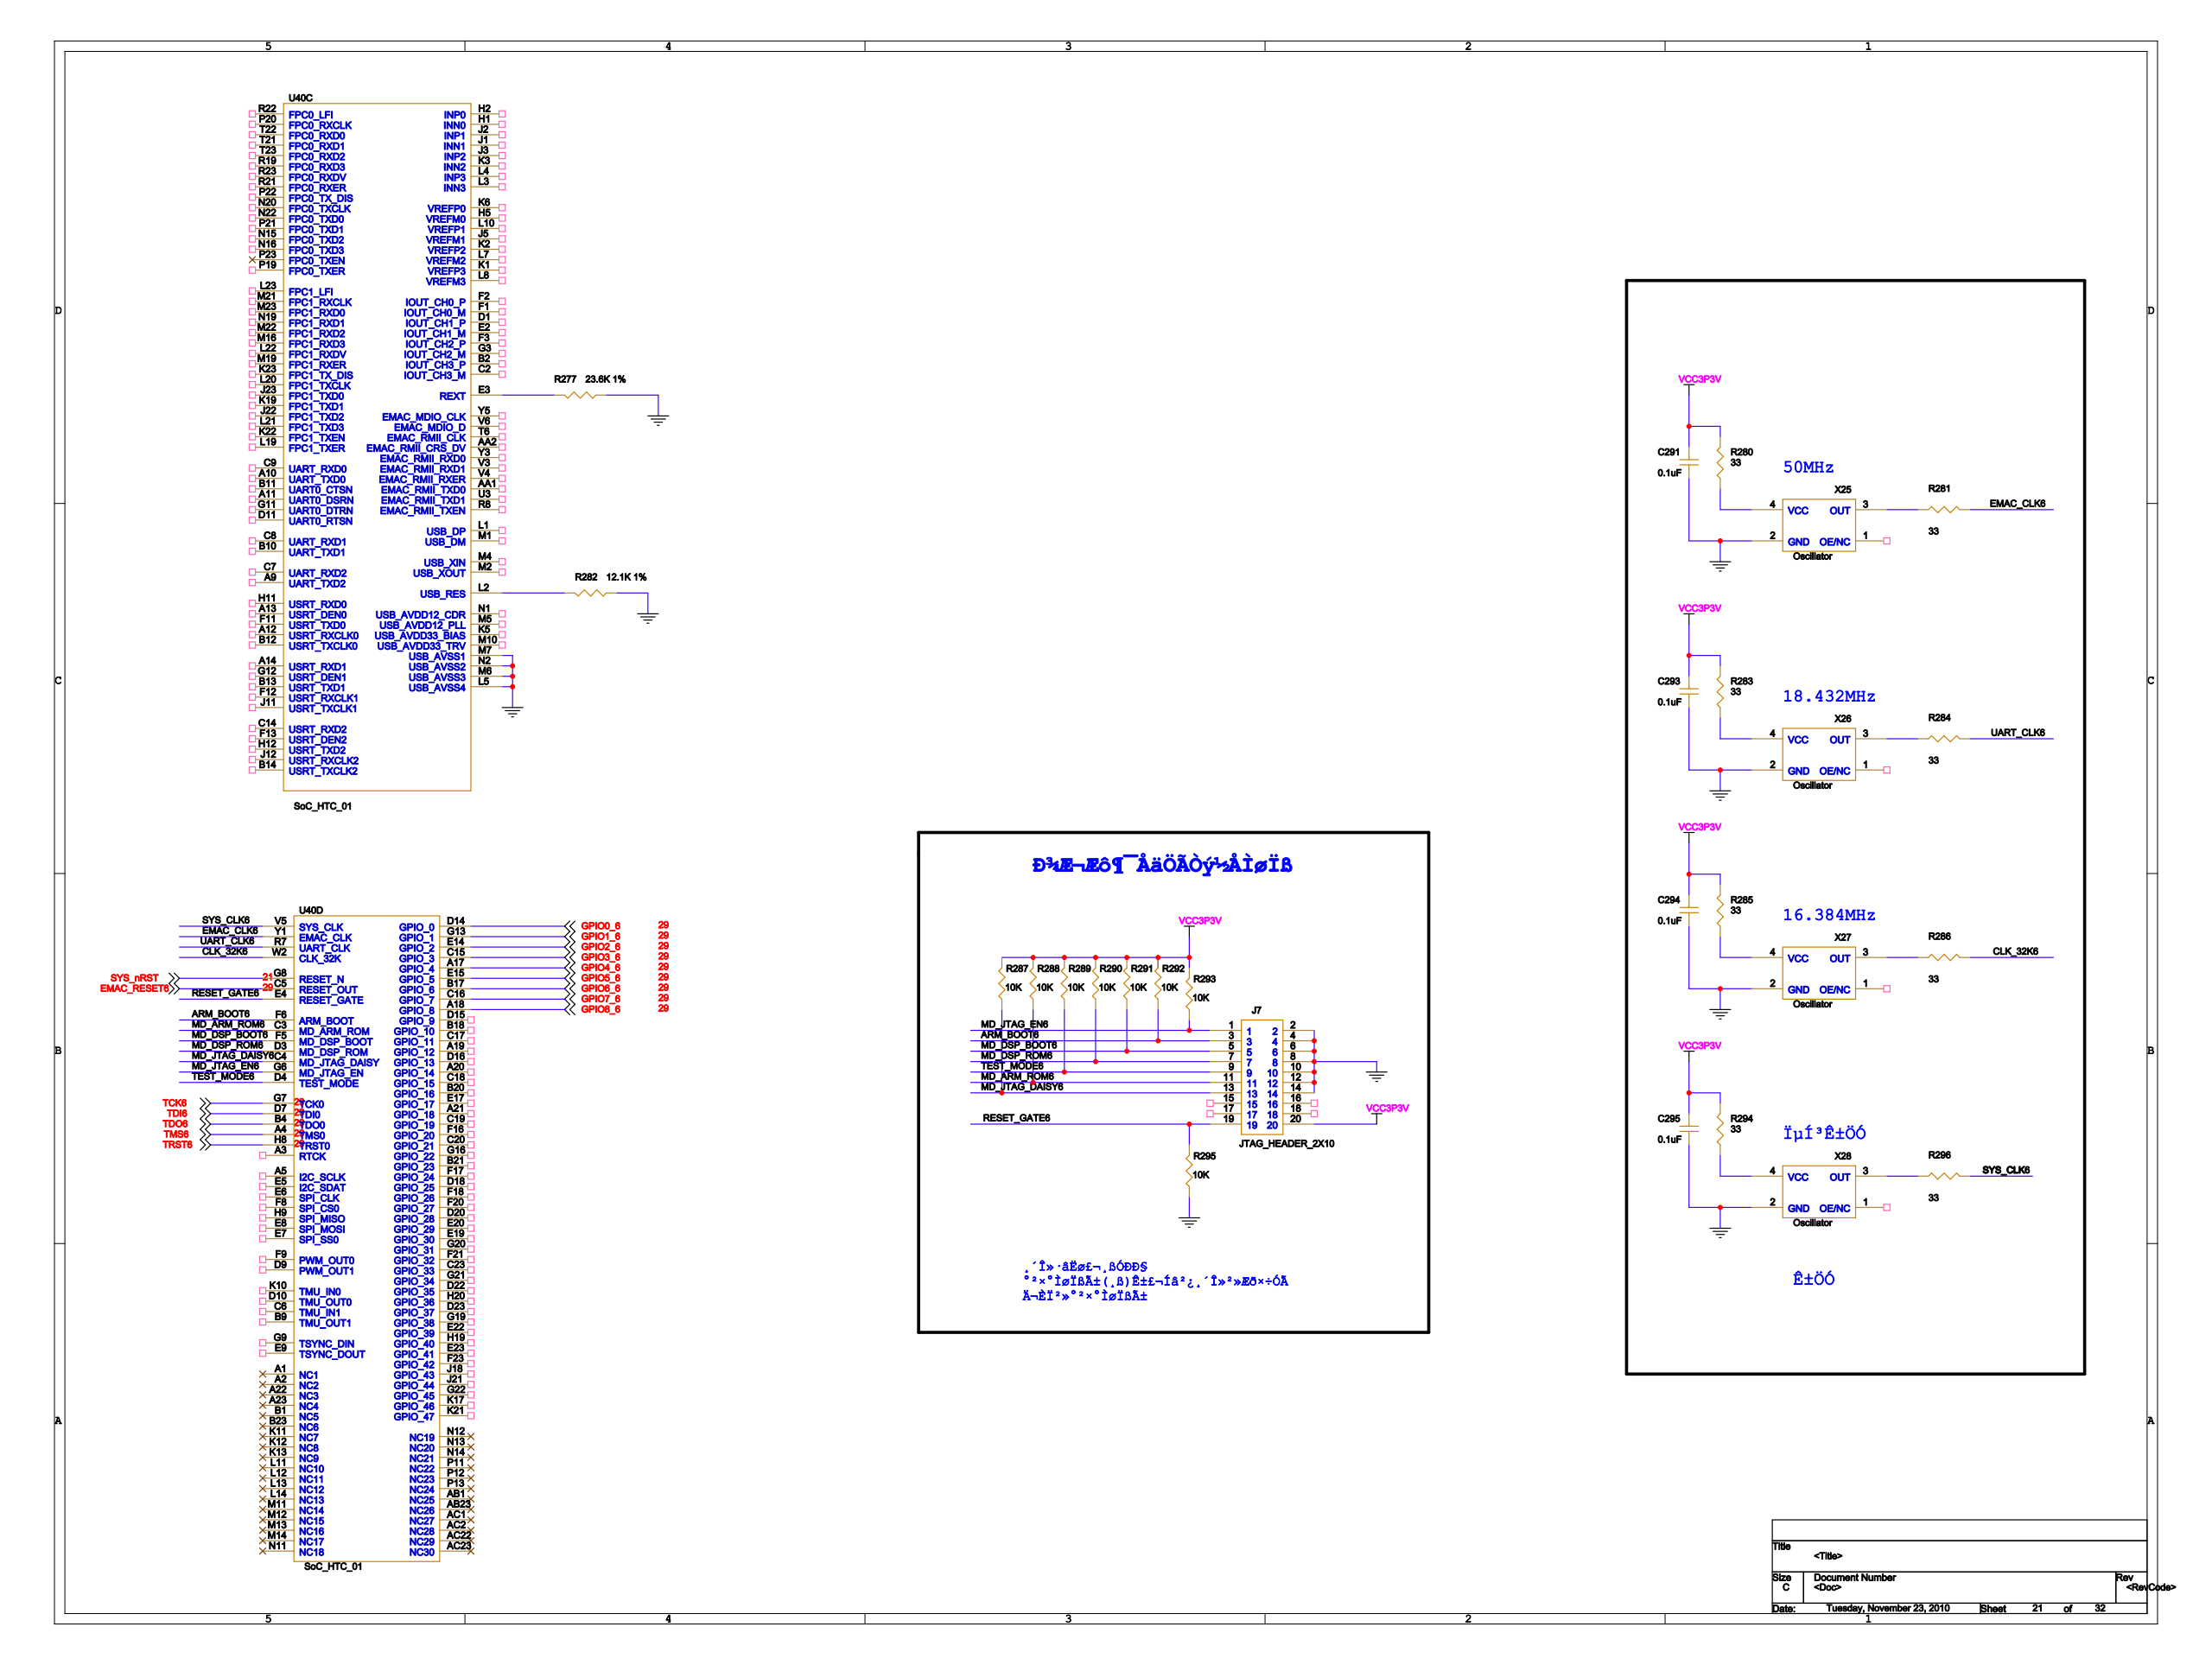Circuit board | Cadence Allegro | 1001 parts | 1318 nets | one sheet of the schematic
Parts on this sheet (reference | value | footprint):
C291 | 0.1uF | 0603
C293 | 0.1uF | 0603
C294 | 0.1uF | 0603
C295 | 0.1uF | 0603
J7 | JTAG_HEADER_2X10 | JTAG_HEADER_2X10
R277 | 23.6K 1% | 0603
R280 | 33 | 0603
R281 | 33 | 0603
R282 | 12.1K 1% | 0603
R283 | 33 | 0603
R284 | 33 | 0603
R285 | 33 | 0603
R286 | 33 | 0603
R287 | 10K | 0603
R288 | 10K | 0603
R289 | 10K | 0603
R290 | 10K | 0603
R291 | 10K | 0603
R292 | 10K | 0603
R293 | 10K | 0603
R294 | 33 | 0603
R295 | 10K | 0603
R296 | 33 | 0603
U40 | SoC_HTC_01 | L529_XIN
X25 | Oscillator | OSC_5_7
X26 | Oscillator | OSC_5_7
X27 | Oscillator | OSC_5_7
X28 | Oscillator | OSC_5_7
Nets of these parts (net: part-pin ...):
EMAC_RESET6: U40-C5
GPIO1_6: U40-G13
TRST6: U40-H8
TDI6: U40-D7
GPIO2_6: U40-E14
TDO6: U40-B4
TMS6: U40-A4
GPIO8_6: U40-A18
GPIO0_6: U40-D14
GPIO6_6: U40-B17
GPIO4_6: U40-A17
GPIO7_6: U40-C16
GPIO5_6: U40-E15
GPIO3_6: U40-C15
TCK6: U40-G7
GND: C291-2 C293-2 C294-2 C295-2 J7-2 J7-4 J7-6 J7-8 J7-10 J7-12 J7-14 R277-1 R282-1 R295-1 X25-2 X26-2 X27-2 X28-2 U40-L5 U40-M6 U40-M7 U40-N2
VCC3P3V: C291-1 C293-1 C294-1 C295-1 J7-20 R280-2 R283-2 R285-2 R287-2 R288-2 R289-2 R290-2 R291-2 R292-2 R293-2 R294-2 U40-J7
N16917267: R277-2 U40-E3
N16917488: R282-2 U40-L2
ARM_BOOT6: J7-3 R292-1 U40-F6
CLK_32K6: R286-2 U40-W2
EMAC_CLK6: R281-2 U40-Y1
MD_ARM_ROM6: J7-11 R288-1 U40-C3
MD_DSP_BOOT6: J7-5 R291-1 U40-F5
MD_DSP_ROM6: J7-7 R290-1 U40-D3
MD_JTAG_DAISY6: J7-13 R287-1 U40-C4
MD_JTAG_EN6: J7-1 R293-1 U40-G6
RESET_GATE6: J7-19 R295-2 U40-E4
SYS_CLK_16917057: R296-2 U40-V5
TEST_MODE6: J7-9 R289-1 U40-D4
UART_CLK6: R284-2 U40-R7
N16918008: R280-1 X25-4
N16917968: R281-1 X25-3
N16917986: R283-1 X26-4
N16918000: R284-1 X26-3
N16917032: R285-1 X27-4
N16917069: R286-1 X27-3
N16917055: R294-1 X28-4
N16917102: R296-1 X28-3